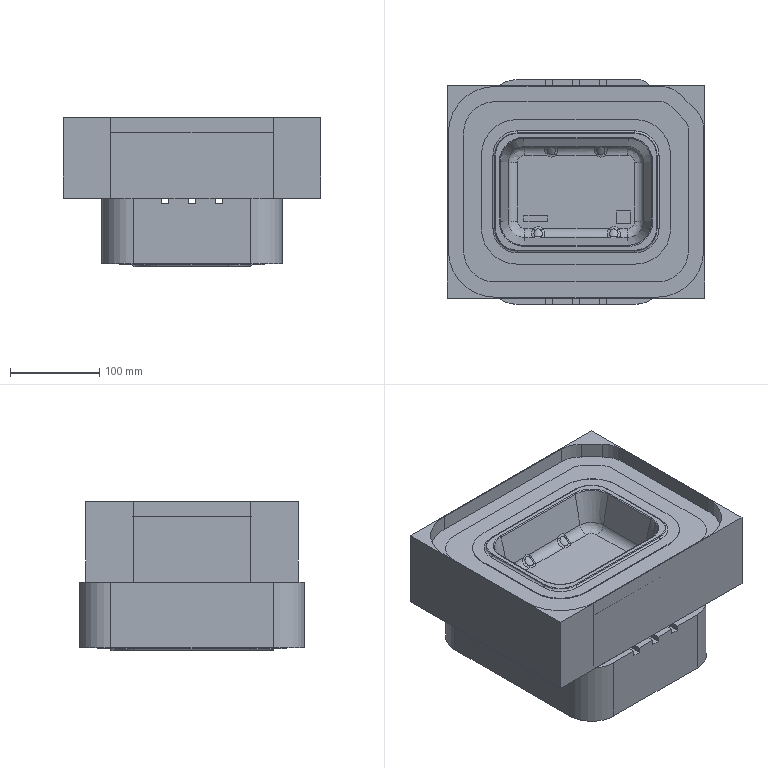NC program | NX | posted with a generic post | part box 287.436 x 251.436 x 167.016 mm
Lines 12631 to 13522 of 118587:
(06 , TOOL : R2)
N25248 M6
N25250 G53
N25252 G17 G0 G90 X-67.849 Y-80.733 S8000 M3 M8
N25254 G43 Z240.5 H0
N25256 Z77.182
N25258 G94 G1 Z74.182 F4500.
N25260 X-69.235 Y-80.679
N25262 X-69.472 Y-80.657
N25264 X-69.58 Y-80.643
N25266 X-70.616 Y-80.526
N25268 X-72.004 Y-80.366
N25270 X-72.391 Y-80.311
N25272 X-74.221 Y-79.965
N25274 X-75.119 Y-79.784
N25276 X-75.413 Y-79.709
N25278 X-75.763 Y-79.619
N25280 X-75.811 Y-79.604
N25282 X-77.051 Y-79.274
N25284 X-77.888 Y-79.04
N25286 X-78.235 Y-78.928
N25288 X-78.245 Y-78.926
N25290 X-80.658 Y-78.075
N25292 X-81.907 Y-77.542
N25294 X-83.423 Y-76.876
N25296 X-83.475 Y-76.849
N25298 X-83.772 Y-76.692
N25300 X-85.849 Y-75.594
N25302 X-86.083 Y-75.464
N25304 X-88.283 Y-74.081
N25306 X-88.617 Y-73.857
N25308 X-88.785 Y-73.734
N25310 X-88.966 Y-73.6
N25312 X-89.258 Y-73.387
N25314 G2 X-96.971 Y-66.118 R37.721
N25316 G1 X-97.247 Y-65.772
N25318 X-97.824 Y-64.992
N25320 X-98.313 Y-64.329
N25322 X-98.78 Y-63.695
N25324 X-99.004 Y-63.36
N25326 X-99.01 Y-63.349
N25328 X-100.389 Y-61.158
N25330 X-100.519 Y-60.924
N25332 X-101.428 Y-59.205
N25334 X-101.799 Y-58.502
N25336 X-102.71 Y-56.425
N25338 X-103. Y-55.733
N25340 X-103.853 Y-53.31
N25342 X-103.965 Y-52.964
N25344 X-104.158 Y-52.277
N25346 X-104.621 Y-50.541
N25348 G2 X-105.291 Y-47.079 R49.648
N25350 G1 X-105.582 Y-44.549
N25352 X-105.601 Y-44.31
N25354 X-105.602 Y-44.28
N25356 X-105.658 Y-42.925
N25358 X-105.706 Y-41.54
N25360 X-105.712 Y-41.194
N25362 X-105.715 Y-40.855
N25364 Y41.187
N25366 X-105.684 Y42.228
N25368 X-105.658 Y42.925
N25370 X-105.602 Y44.28
N25372 X-105.6 Y44.31
N25374 X-105.582 Y44.547
N25376 X-105.568 Y44.656
N25378 X-105.451 Y45.693
N25380 X-105.291 Y47.079
N25382 X-105.236 Y47.466
N25384 X-104.89 Y49.296
N25386 X-104.781 Y49.847
N25388 X-104.709 Y50.194
N25390 X-104.634 Y50.488
N25392 X-104.544 Y50.838
N25394 X-104.343 Y51.579
N25396 X-104.067 Y52.616
N25398 X-103.968 Y52.956
N25400 X-103.853 Y53.31
N25402 X-103.851 Y53.321
N25404 X-103. Y55.733
N25406 X-102.256 Y57.464
N25408 X-101.801 Y58.498
N25410 X-101.774 Y58.55
N25412 X-101.617 Y58.848
N25414 X-100.519 Y60.924
N25416 X-100.389 Y61.158
N25418 X-100.317 Y61.272
N25420 X-100.042 Y61.709
N25422 X-99.448 Y62.656
N25424 X-99.006 Y63.358
N25426 X-98.782 Y63.692
N25428 X-98.659 Y63.86
N25430 X-98.313 Y64.33
N25432 X-98.27 Y64.387
N25434 X-98.077 Y64.649
N25436 X-97.251 Y65.768
N25438 X-96.928 Y66.172
N25440 X-95.186 Y68.195
N25442 X-93.109 Y70.272
N25444 X-91.043 Y72.046
N25446 X-90.664 Y72.349
N25448 X-90.35 Y72.581
N25450 X-88.62 Y73.855
N25452 X-88.284 Y74.079
N25454 X-88.274 Y74.085
N25456 X-87.184 Y74.772
N25458 X-86.635 Y75.118
N25460 X-86.083 Y75.464
N25462 X-85.849 Y75.594
N25464 X-84.13 Y76.503
N25466 X-83.427 Y76.874
N25468 X-81.112 Y77.888
N25470 X-80.658 Y78.075
N25472 X-80.066 Y78.287
N25474 X-78.235 Y78.928
N25476 X-77.888 Y79.04
N25478 X-77.055 Y79.272
N25480 X-75.465 Y79.696
N25482 G2 X-72.004 Y80.366 R49.649
N25484 G1 X-69.473 Y80.657
N25486 X-69.234 Y80.676
N25488 X-67.849 Y80.733
N25490 X-66.465 Y80.781
N25492 X-66.119 Y80.79
N25494 X66.119 Y80.786
N25496 X66.459 Y80.779
N25498 X67.153 Y80.759
N25500 X67.849 Y80.733
N25502 X69.204 Y80.677
N25504 X69.234 Y80.675
N25506 X69.472 Y80.657
N25508 X69.58 Y80.643
N25510 X70.617 Y80.526
N25512 X72.004 Y80.366
N25514 X72.391 Y80.311
N25516 X74.771 Y79.856
N25518 X75.119 Y79.784
N25520 X75.413 Y79.709
N25522 X75.763 Y79.619
N25524 G2 X80.658 Y78.075 R36.873
N25526 G1 X81.112 Y77.888
N25528 X83.475 Y76.849
N25530 X83.773 Y76.692
N25532 X84.787 Y76.156
N25534 X85.849 Y75.594
N25536 X86.082 Y75.465
N25538 X88.283 Y74.081
N25540 X88.617 Y73.857
N25542 X88.785 Y73.734
N25544 X90.675 Y72.34
N25546 X91.096 Y72.003
N25548 X93.109 Y70.272
N25550 X95.186 Y68.195
N25552 X96.971 Y66.118
N25554 X97.051 Y66.018 Z74.18
N25556 X97.246 Y65.773 Z74.182
N25558 X98.313 Y64.329
N25560 X98.78 Y63.695
N25562 X99.004 Y63.36
N25564 X99.01 Y63.349
N25566 X100.389 Y61.158
N25568 X100.518 Y60.926
N25570 X100.882 Y60.234
N25572 X101.066 Y59.887
N25574 X101.799 Y58.502
N25576 X102.256 Y57.464
N25578 X103. Y55.733
N25580 G2 X104.709 Y50.194 R41.459
N25582 G1 X104.78 Y49.848
N25584 X104.917 Y49.156
N25586 X105.242 Y47.425
N25588 X105.291 Y47.079
N25590 X105.582 Y44.549
N25592 X105.601 Y44.31
N25594 X105.658 Y42.925
N25596 X105.684 Y42.232
N25598 X105.715 Y41.194
N25600 X105.712 Y-41.194
N25602 X105.706 Y-41.539
N25604 X105.658 Y-42.925
N25606 X105.602 Y-44.28
N25608 X105.6 Y-44.31
N25610 X105.582 Y-44.547
N25612 X105.568 Y-44.656
N25614 X105.451 Y-45.692
N25616 X105.293 Y-47.065
N25618 X105.242 Y-47.425
N25620 X104.917 Y-49.155
N25622 X104.849 Y-49.502
N25624 X104.709 Y-50.194
N25626 X104.634 Y-50.488
N25628 X104.544 Y-50.838
N25630 X104.529 Y-50.887
N25632 X104.199 Y-52.126
N25634 X103.965 Y-52.964
N25636 X103.853 Y-53.31
N25638 X103.851 Y-53.321
N25640 X103. Y-55.733
N25642 X102.813 Y-56.187
N25644 X101.774 Y-58.55
N25646 X101.617 Y-58.848
N25648 X100.519 Y-60.924
N25650 X100.39 Y-61.157
N25652 X100.317 Y-61.272
N25654 X99.005 Y-63.358
N25656 X98.782 Y-63.692
N25658 X98.659 Y-63.86
N25660 X97.265 Y-65.75
N25662 X97.051 Y-66.018 Z74.18
N25664 X96.971 Y-66.118 Z74.182
N25666 X95.197 Y-68.184
N25668 X93.12 Y-70.261
N25670 X91.097 Y-72.002
N25672 X90.697 Y-72.322
N25674 X89.312 Y-73.344
N25676 X89.307 Y-73.349
N25678 X88.62 Y-73.855
N25680 X88.284 Y-74.08
N25682 X86.083 Y-75.464
N25684 X85.85 Y-75.593
N25686 X85.504 Y-75.777
N25688 X84.13 Y-76.503
N25690 X83.427 Y-76.874
N25692 X82.389 Y-77.331
N25694 X80.658 Y-78.075
N25696 G2 X75.119 Y-79.784 R39.779
N25698 G1 X74.773 Y-79.855
N25700 X74.224 Y-79.964
N25702 X72.393 Y-80.311
N25704 X72.004 Y-80.366
N25706 X69.473 Y-80.657
N25708 X69.234 Y-80.676
N25710 X67.849 Y-80.733
N25712 X67.157 Y-80.759
N25714 X66.465 Y-80.779
N25716 X66.119 Y-80.786
N25718 X-66.112 Y-80.79
N25720 X-66.464 Y-80.781
N25722 X-67.849 Y-80.733
N25724 Y-80.657
N25726 Y-80.447
N25728 X-69.287 Y-80.387
N25730 G2 X-80.658 Y-77.765 R40.675
N25732 X-83.427 Y-76.552 R99.899
N25734 G1 X-85.484 Y-75.465
N25736 X-85.723 Y-75.337
N25738 X-85.85 Y-75.267
N25740 X-85.923 Y-75.227
N25742 G2 X-97.06 Y-65.546 R39.317
N25744 X-101.573 Y-58.302 R39.773
N25746 X-103.766 Y-52.618 R38.865
N25748 G1 X-103.86 Y-52.285
N25750 X-103.943 Y-51.979
N25752 X-104.414 Y-50.194
N25754 X-104.62 Y-49.187
N25756 G2 X-105.372 Y-42.925 R34.123
N25758 G1 X-105.428 Y-41.194
N25760 Y41.194
N25762 X-105.372 Y42.925
N25764 X-105.31 Y44.361
N25766 G2 X-104.954 Y47.425 R61.949
N25768 X-102.597 Y55.948 R40.067
N25770 G1 X-102.094 Y57.118
N25772 X-101.897 Y57.573
N25774 X-101.639 Y58.156
N25776 X-101.531 Y58.4
N25778 X-100.192 Y60.926
N25780 X-100.152 Y60.999
N25782 X-100.043 Y61.172
N25784 G2 X-90.472 Y72.136 R39.166
N25786 X-83.325 Y76.606 R39.555
N25788 X-77.236 Y78.926 R39.766
N25790 X-69.151 Y80.394 R40.837
N25792 G1 X-66.811 Y80.484
N25794 X-66.119 Y80.503
N25796 X66.119
N25798 X67.849 Y80.447
N25800 X69.285 Y80.385
N25802 X69.566 Y80.358
N25804 X70.554 Y80.247
N25806 G2 X76.386 Y79.155 R33.785
N25808 X91.043 Y71.673 R38.456
N25810 G1 X92.915 Y70.062
N25812 G2 X101.944 Y57.464 R38.892
N25814 X104.668 Y48.934 R37.469
N25816 G1 X104.951 Y47.433
N25818 G2 X105.314 Y44.31 R106.611
N25820 G1 X105.404 Y42.054
N25822 X105.429 Y41.041
N25824 X105.428 Y-41.194
N25826 X105.372 Y-42.925
N25828 G2 X103.957 Y-51.925 R36.711
N25830 X101.531 Y-58.4 R36.331
N25832 G1 X100.192 Y-60.926
N25834 X100.152 Y-60.998
N25836 X100.043 Y-61.172
N25838 G2 X94.987 Y-67.99 R42.454
N25840 X83.325 Y-76.606 R39.553
N25842 G1 X82.088 Y-77.15
N25844 G2 X74.112 Y-79.695 R37.012
N25846 X70.7 Y-80.23 R26.407
N25848 G1 X69.58 Y-80.357
N25850 X69.151 Y-80.394
N25852 X66.99 Y-80.478
N25854 X66.276 Y-80.5
N25856 X66.119 Y-80.503
N25858 X-66.119
N25860 X-67.849 Y-80.447
N25862 X-67.839 Y-80.162
N25864 X-69.038 Y-80.115
N25866 X-69.234 Y-80.102
N25868 G2 X-81.796 Y-76.968 R38.488
N25870 X-92.709 Y-69.861 R38.141
N25872 G1 X-94.724 Y-67.849
N25874 G2 X-105.025 Y-44.31 R38.878
N25876 G1 X-105.073 Y-43.271
N25878 X-105.138 Y-41.442
N25880 X-105.145 Y-40.848
N25882 X-105.141 Y41.289
N25884 X-105.087 Y42.925
N25886 G2 X-102.547 Y55.306 R37.867
N25888 X-101.234 Y58.35 R77.91
N25890 X-88.285 Y73.388 R38.937
N25892 X-83.275 Y76.309 R45.716
N25894 G1 X-83.081 Y76.4
N25896 G2 X-67.645 Y80.169 R38.524
N25898 G1 X-66.119 Y80.218
N25900 X66.119
N25902 X67.849 Y80.162
N25904 G2 X76.85 Y78.736 R36.853
N25906 X103.552 Y52.333 R38.75
N25908 G1 X104.12 Y50.194
N25910 G2 X104.734 Y46.923 R63.626
N25912 G1 X105.016 Y44.435
N25914 X105.044 Y43.963
N25916 X105.117 Y42.113
N25918 X105.144 Y41.102
N25920 X105.142 Y-41.288
N25922 X105.081 Y-43.08
N25924 G2 X103.25 Y-53.31 R37.587
N25926 X91.043 Y-71.297 R38.665
N25928 X86.111 Y-74.772 R36.949
N25930 X66.927 Y-80.195 R38.668
N25932 G1 X66.213 Y-80.216
N25934 X66.119 Y-80.218
N25936 X-66.119
N25938 X-67.839 Y-80.162
N25940 X-67.828 Y-79.878
N25942 G2 X-77.591 Y-78.234 R37.518
N25944 X-83.033 Y-76.109 R41.774
N25946 G1 X-83.427 Y-75.907
N25948 X-85.566 Y-74.772
N25950 X-86.543 Y-74.166
N25952 G2 X-92.507 Y-69.659 R36.951
N25954 X-104.805 Y-42.84 R38.466
N25956 G1 X-104.85 Y-41.54
N25958 X-104.859 Y-41.163
N25960 X-104.858 Y41.226
N25962 G2 X-104.725 Y44.474 R55.749
N25964 X-100.832 Y58.502 R38.885
N25966 G1 X-100.043 Y59.994
N25968 X-99.769 Y60.508
N25970 G2 X-85.85 Y74.596 R38.533
N25972 G1 X-85.559 Y74.772
N25974 X-84.692 Y75.239
N25976 G2 X-71.741 Y79.535 R38.091
N25978 X-66.15 Y79.933 R39.099
N25980 G1 X66.088 Y79.934
N25982 X67.765 Y79.88
N25984 G2 X81.004 Y77.001 R37.717
N25986 X96.633 Y65.164 R38.415
N25988 X104.849 Y41.54 R38.518
N25990 G1 X104.859 Y41.163
N25992 X104.858 Y-41.225
N25994 G2 X104.725 Y-44.474 R56.006
N25996 X94.65 Y-67.503 R38.628
N25998 X82.93 Y-76.157 R38.846
N26000 X80.165 Y-77.342 R59.985
N26002 X70.621 Y-79.665 R37.301
N26004 G1 X69.399 Y-79.8
N26006 X68.888 Y-79.834
N26008 X66.864 Y-79.912
N26010 X66.15 Y-79.933
N26012 X-66.088 Y-79.934
N26014 X-67.828 Y-79.878
N26016 X-67.824 Y-79.593
N26018 X-69.153 Y-79.538
N26020 G2 X-78.88 Y-77.495 R37.939
N26022 X-81.617 Y-76.424 R24.696
N26024 G1 X-82.791 Y-75.908
N26026 G2 X-104.432 Y-44.544 R38.287
N26028 G1 X-104.454 Y-44.31
N26030 G2 X-104.573 Y-41.228 R81.56
N26032 G1 X-104.574 Y41.161
N26034 X-104.516 Y42.953
N26036 G2 X-99.466 Y60.464 R38.026
N26038 X-92.428 Y69.337 R39.433
N26040 X-82.518 Y76.028 R38.559
N26042 X-76.972 Y78.112 R37.513
N26044 X-68.888 Y79.549 R38.68
N26046 G1 X-67.877 Y79.591
N26048 X-66.468 Y79.64
N26050 X-66.122 Y79.649
N26052 X66.116
N26054 X67.13 Y79.619
N26056 X67.823 Y79.593
N26058 X69.234 Y79.529
N26060 X70.403 Y79.403
N26062 G2 X80.637 Y76.849 R38.111
N26064 X90.426 Y71.074 R37.642
N26066 X100.82 Y57.895 R38.309
N26068 G1 X101.131 Y57.189
N26070 G2 X103.821 Y48.81 R36.406
N26072 X104.543 Y42.232 R33.916
N26074 G1 X104.573 Y41.227
N26076 X104.574 Y-41.16
N26078 G2 X104.446 Y-44.407 R105.003
N26080 X99.399 Y-60.579 R38.364
N26082 X87.581 Y-73.171 R38.554
N26084 G1 X87.244 Y-73.388
N26086 G2 X81.901 Y-76.299 R36.558
N26088 X70.619 Y-79.378 R37.287
N26090 G1 X69.332 Y-79.521
N26092 X68.888 Y-79.549
N26094 X67.877 Y-79.591
N26096 X67.158 Y-79.618
N26098 X66.122 Y-79.649
N26100 X-66.116
N26102 X-66.462 Y-79.64
N26104 X-67.824 Y-79.593
N26106 X-67.814 Y-79.308
N26108 X-69.21 Y-79.249
N26110 G2 X-80.423 Y-76.626 R39.314
N26112 G1 X-81.366 Y-76.222
N26114 G2 X-90.112 Y-70.964 R36.934
N26116 X-103.801 Y-47.375 R38.037
N26118 X-104.188 Y-43.963 R39.154
N26120 G1 X-104.23 Y-42.962
N26122 X-104.288 Y-41.194
N26124 X-104.287 Y41.194
N26126 X-104.233 Y42.888
N26128 G2 X-101.464 Y55.697 R37.16
N26130 X-93.812 Y67.553 R37.792
N26132 X-91.043 Y70.168 R27.966
N26134 X-77.89 Y77.54 R37.512
N26136 X-74.132 Y78.529 R46.194
N26138 X-66.811 Y79.343 R37.273
N26140 G1 X-66.027 Y79.364
N26142 X66.207 Y79.361
N26144 X67.157 Y79.332
N26146 X67.847 Y79.306
N26148 X69.234 Y79.245
N26150 G2 X97.62 Y62.861 R38.026
N26152 X102.465 Y52.964 R38.023
N26154 X104.172 Y44.284 R40.352
N26156 G1 X104.255 Y42.293
N26158 X104.287 Y41.194
N26160 X104.288 Y-41.194
N26162 X104.233 Y-42.888
N26164 G2 X103.32 Y-49.848 R36.948
N26166 X97.62 Y-62.852 R38.672
N26168 X80.622 Y-76.539 R37.73
N26170 X71.659 Y-78.971 R37.32
N26172 G1 X70.823 Y-79.068
N26174 X69.234 Y-79.244
N26176 X68.897 Y-79.263
N26178 X67.852 Y-79.306
N26180 X67.157 Y-79.333
N26182 X66.027 Y-79.364
N26184 X-66.208 Y-79.361
N26186 X-66.544 Y-79.352
N26188 X-67.814 Y-79.308
N26190 X-67.804 Y-79.023
N26192 X-68.887 Y-78.98
N26194 X-69.232 Y-78.96
N26196 G2 X-82.384 Y-75.465 R37.853
N26198 G1 X-82.624 Y-75.354
N26200 X-83.081 Y-75.123
N26202 G2 X-87.64 Y-72.449 R38.115
N26204 X-103.502 Y-47.425 R37.676
N26206 X-104. Y-41.342 R38.89
N26208 G1 X-104.004 Y-39.183
N26210 X-104.002 Y41.194
N26212 X-103.95 Y42.826
N26214 X-103.906 Y43.909
N26216 G2 X-103.091 Y49.57 R37.858
N26218 X-71.936 Y78.648 R37.729
N26220 X-67.849 Y79.021 R34.091
N26222 G1 X-66.675 Y79.062
N26224 X-65.966 Y79.079
N26226 X66.119 Y79.077
N26228 X67.849 Y79.021
N26230 G2 X72.004 Y78.637 R29.727
N26232 X101.52 Y54.798 R37.727
N26234 X103.903 Y43.963 R38.841
N26236 G1 X103.979 Y42.014
N26238 X104.004 Y41.
N26240 X104.002 Y-41.194
N26242 X103.95 Y-42.826
N26244 G2 X103.562 Y-47.079 R34.249
N26246 X93.812 Y-67.145 R37.913
N26248 X82.394 Y-75.46 R38.484
N26250 X71.936 Y-78.648 R37.859
N26252 X68.889 Y-78.978 R43.378
N26254 G1 X67.032 Y-79.051
N26256 X65.966 Y-79.079
N26258 X-66.119 Y-79.077
N26260 X-67.804 Y-79.023
N26262 X-67.794 Y-78.738
N26264 G2 X-73.734 Y-78.025 R31.327
N26266 G1 X-74.081 Y-77.957
N26268 X-74.773 Y-77.811
N26270 G2 X-82.459 Y-75.118 R38.43
N26272 X-103.713 Y-41.402 R37.457
N26274 G1 X-103.718 Y-41.194
N26276 X-103.719 Y-41.062
N26278 X-103.718 Y41.194
N26280 X-103.667 Y42.763
N26282 G2 X-101.251 Y54.695 R36.677
N26284 X-82.45 Y75.118 R37.518
N26286 X-68.77 Y78.698 R38.049
N26288 G1 X-67.849 Y78.736
N26290 X-66.465 Y78.784
N26292 X-65.905 Y78.794
N26294 X66.119 Y78.793
N26296 X67.849 Y78.736
N26298 G2 X74.426 Y77.888 R32.705
N26300 X100.043 Y57.535 R37.411
N26302 G1 X100.53 Y56.425
N26304 G2 X103.687 Y42.232 R36.678
N26306 G1 X103.719 Y41.062
N26308 X103.715 Y-41.33
N26310 G2 X103.567 Y-44.593 R79.654
N26312 X82.334 Y-75.173 R37.389
N26314 G1 X81.35 Y-75.605
N26316 G2 X67.157 Y-78.762 R37.124
N26318 G1 X66.255 Y-78.79
N26320 X66.119 Y-78.793
N26322 X-66.119
N26324 X-67.794 Y-78.738
N26326 X-67.783 Y-78.453
N26328 G2 X-77.729 Y-76.69 R35.996
N26330 G1 X-79.619 Y-76.023
N26332 X-80.022 Y-75.867
N26334 X-81.233 Y-75.347
N26336 G2 X-89.658 Y-70.23 R36.563
N26338 G1 X-91.498 Y-68.65
N26340 G2 X-103.412 Y-41.886 R37.175
N26342 G1 X-103.434 Y-41.123
N26344 X-103.431 Y41.268
N26346 X-103.384 Y42.699
N26348 G2 X-100.353 Y56.116 R36.296
N26350 X-91.389 Y68.736 R36.847
N26352 X-69.071 Y78.397 R37.292
N26354 G1 X-67.625 Y78.459
N26356 X-66.119 Y78.508
N26358 X66.119
N26360 X67.849 Y78.45
N26362 G2 X82.888 Y74.58 R36.659
N26364 X102.377 Y50.104 R36.976
N26366 G1 X102.442 Y49.848
N26368 X102.467 Y49.75
N26370 G2 X103.402 Y42.232 R36.493
N26372 G1 X103.434 Y41.122
N26374 X103.432 Y-41.267
N26376 X103.375 Y-42.925
N26378 G2 X102.436 Y-49.879 R36.895
N26380 X82.276 Y-74.885 R37.19
N26382 G1 X81.35 Y-75.294
N26384 G2 X67.264 Y-78.473 R36.499
N26386 G1 X66.119 Y-78.508
N26388 X-66.119
N26390 X-67.783 Y-78.453
N26392 Y-78.168
N26394 G2 X-73.942 Y-77.403 R31.517
N26396 X-81.003 Y-75.136 R35.593
N26398 X-94.812 Y-64.694 R36.447
N26400 G1 X-94.963 Y-64.516
N26402 G2 X-103.09 Y-42.925 R36.737
N26404 G1 X-103.139 Y-41.54
N26406 X-103.149 Y-41.194
N26408 X-103.148 Y41.205
N26410 G2 X-103.008 Y44.46 R86.936
N26412 X-102.229 Y49.502 R38.617
N26414 X-99.602 Y57.118 R37.192
N26416 X-87.157 Y71.735 R36.838
N26418 X-77.618 Y76.427 R36.436
N26420 X-75.204 Y77.111 R26.715
N26422 G1 X-74.734 Y77.234
N26424 G2 X-68.643 Y78.133 R36.077
N26426 G1 X-67.849 Y78.165
N26428 X-66.485 Y78.214
N26430 X-66.119 Y78.224
N26432 X66.108
N26434 X67.116 Y78.193
N26436 X67.783 Y78.168
N26438 G2 X82.418 Y74.504 R36.718
N26440 X103.117 Y42.232 R36.785
N26442 G1 X103.148 Y41.194
N26444 X103.149 Y-41.194
N26446 X103.139 Y-41.54
N26448 X103.101 Y-42.637
N26450 G2 X102.159 Y-49.809 R36.984
N26452 X67.201 Y-78.19 R36.824
N26454 G1 X66.129 Y-78.223
N26456 X-66.108 Y-78.224
N26458 X-66.446 Y-78.215
N26460 X-67.783 Y-78.168
N26462 X-67.773 Y-77.883
N26464 G2 X-79.273 Y-75.543 R35.553
N26466 G1 X-79.487 Y-75.465
N26468 X-79.619 Y-75.413
N26470 X-80.658 Y-74.975
N26472 G2 X-101.854 Y-49.848 R36.401
N26474 X-102.805 Y-42.925 R34.76
N26476 G1 X-102.863 Y-41.194
N26478 Y41.194
N26480 X-102.819 Y42.572
N26482 G2 X-93.466 Y65.823 R36.441
N26484 X-67.857 Y77.88 R36.454
N26486 G1 X-66.467 Y77.929
N26488 X-66.12 Y77.939
N26490 X66.117 Y77.938
N26492 G2 X69.234 Y77.812 R50.755
N26494 X101.326 Y51.823 R36.562
N26496 X102.831 Y42.254 R35.758
N26498 G1 X102.862 Y41.246
N26500 X102.863 Y41.194
N26502 Y-41.194
N26504 G2 X102.729 Y-44.394 R97.577
N26506 X101.937 Y-49.502 R36.746
N26508 X96.255 Y-62.31 R36.8
N26510 X93.466 Y-65.823 R34.695
N26512 X79.152 Y-75.586 R36.834
N26514 X67.16 Y-77.906 R36.508
N26516 G1 X66.12 Y-77.938
N26518 X-66.117
N26520 X-66.462 Y-77.929
N26522 X-67.773 Y-77.883
N26524 X-67.764 Y-77.598
N26526 G2 X-71.98 Y-77.195 R28.768
N26528 X-88.665 Y-69.926 R36.463
N26530 X-102.52 Y-42.925 R36.147
N26532 G1 X-102.577 Y-41.194
N26534 Y41.194
N26536 X-102.536 Y42.509
N26538 G2 X-92.815 Y66.118 R36.199
N26540 X-68.89 Y77.551 R36.399
N26542 G1 X-67.851 Y77.595
N26544 X-66.718 Y77.635
N26546 X-66.007 Y77.653
N26548 X66.119 Y77.652
N26550 X67.848 Y77.595
N26552 G2 X79.335 Y75.217 R35.426
N26554 X99.005 Y57.059 R36.173
N26556 X100.166 Y54.348 R53.776
N26558 X102.546 Y42.232 R35.771
N26560 G1 X102.575 Y41.302
N26562 X102.577 Y41.194
N26564 Y-41.194
N26566 G2 X102.449 Y-44.327 R66.803
N26568 X101.644 Y-49.502 R36.419
N26570 X68.89 Y-77.551 R36.281
N26572 G1 X67.851 Y-77.595
N26574 X67.157 Y-77.621
N26576 X66.007 Y-77.653
N26578 X-66.227 Y-77.65
N26580 X-66.465 Y-77.643
N26582 X-67.764 Y-77.598
N26584 X-67.753 Y-77.313
N26586 G2 X-77.087 Y-75.701 R35.081
N26588 X-102.189 Y-43.963 R35.976
N26590 G1 X-102.243 Y-42.701
N26592 X-102.292 Y-41.194
N26594 X-102.291 Y41.194
N26596 X-102.253 Y42.446
N26598 G2 X-93.055 Y65.426 R35.878
N26600 X-68.814 Y77.269 R36.069
N26602 G1 X-67.849 Y77.31
N26604 X-67.372 Y77.327
N26606 X-66.119 Y77.367
N26608 X66.119 Y77.366
N26610 X67.849 Y77.309
N26612 G2 X84.12 Y72.637 R35.716
N26614 X102.267 Y42.033 R35.938
N26616 G1 X102.293 Y41.02
N26618 X102.292 Y-41.194
N26620 X102.252 Y-42.447
N26622 G2 X100.825 Y-51.49 R34.902
N26624 X67.012 Y-77.341 R35.963
N26626 G1 X65.946 Y-77.368
N26628 X-66.119 Y-77.367
N26630 X-67.753 Y-77.313
N26632 X-67.743 Y-77.028
N26634 G2 X-80.658 Y-74.042 R34.988
N26636 X-101.275 Y-48.464 R35.613
N26638 X-101.955 Y-42.76 R31.107
N26640 G1 X-102.007 Y-41.194
N26642 X-102.004 Y41.31
N26644 G2 X-101.876 Y44.31 R90.531
N26646 X-66.591 Y77.069 R35.708
N26648 G1 X-65.885 Y77.083
N26650 X66.119 Y77.081
N26652 X67.849 Y77.024
N26654 G2 X79.775 Y74.426 R35.182
N26656 X99.774 Y53.748 R35.534
N26658 X101.98 Y42.092 R35.907
N26660 G1 X102.008 Y41.081
N26662 X102.005 Y-41.309
N26664 G2 X98.335 Y-57.117 R35.854
N26666 X66.949 Y-77.057 R35.686
N26668 G1 X66.235 Y-77.079
N26670 X66.119 Y-77.081
N26672 X-66.119 Y-77.082
N26674 X-67.743 Y-77.028
N26676 X-67.733 Y-76.743
N26678 G2 X-81.847 Y-73.192 R35.173
N26680 X-92.428 Y-65.283 R35.493
N26682 X-95.712 Y-61.094 R36.01
N26684 X-101.664 Y-42.925 R35.248
N26686 G1 X-101.723 Y-41.143
N26688 X-101.721 Y41.247
N26690 X-101.701 Y41.886
N26692 G2 X-68.687 Y76.704 R35.413
N26694 G1 X-67.849 Y76.739
N26696 X-66.119 Y76.798
N26698 X66.119 Y76.797
N26700 G2 X71.311 Y76.427 R37.706
N26702 X101.701 Y41.886 R35.366
N26704 G1 X101.722 Y41.194
N26706 X101.723 Y41.143
N26708 X101.722 Y-41.247
N26710 G2 X100.777 Y-49.461 R37.559
N26712 X67.157 Y-76.766 R35.415
N26714 G1 X66.172 Y-76.796
N26716 X66.119 Y-76.797
N26718 X-66.119
N26720 X-66.465 Y-76.788
N26722 X-67.733 Y-76.743
N26724 X-67.723 Y-76.459
N26726 G2 X-71.6 Y-76.1 R33.297
N26728 X-93.707 Y-63.349 R35.3
N26730 X-101.428 Y-41.54 R35.324
N26732 G1 X-101.438 Y-41.194
N26734 Y41.183
N26736 X-101.416 Y41.886
N26738 G2 X-67.849 Y76.454 R35.102
N26740 G1 X-66.467 Y76.503
N26742 X-66.12 Y76.513
N26744 X66.117
N26746 X67.135 Y76.481
N26748 G2 X100.975 Y46.971 R35.07
N26750 X101.405 Y42.232 R35.119
N26752 G1 X101.437 Y41.205
N26754 X101.438 Y-41.182
N26756 X101.364 Y-43.271
N26758 G2 X93.466 Y-63.631 R34.957
N26760 X67.181 Y-76.48 R35.069
N26762 G1 X66.12 Y-76.513
N26764 X-66.117
N26766 X-66.463 Y-76.503
N26768 X-67.723 Y-76.459
N26770 X-67.713 Y-76.174
N26772 G2 X-71.607 Y-75.811 R34.352
N26774 G1 X-71.946 Y-75.753
N26776 G2 X-88.204 Y-68.471 R34.839
N26778 X-101.093 Y-42.939 R34.849
N26780 G1 X-101.152 Y-41.194
N26782 Y41.194
N26784 X-101.133 Y41.835
N26786 G2 X-67.852 Y76.169 R34.817
N26788 G1 X-66.048 Y76.228
N26790 X66.178 Y76.225
N26792 G2 X69.234 Y76.092 R73.05
N26794 X100.677 Y47.02 R34.826
N26796 X101.119 Y42.269 R31.472
N26798 G1 X101.15 Y41.263
N26800 X101.152 Y41.194
N26802 Y-41.194
N26804 X101.082 Y-43.191
N26806 G2 X67.16 Y-76.195 R34.815
N26808 G1 X66.048 Y-76.228
N26810 X-66.187 Y-76.226
N26812 X-66.465 Y-76.218
N26814 X-67.713 Y-76.174
N26816 X-67.703 Y-75.889
N26818 G2 X-81.004 Y-72.645 R34.341
N26820 X-100.808 Y-42.925 R34.515
N26822 G1 X-100.866 Y-41.194
N26824 Y41.194
N26826 X-100.838 Y42.131
N26828 G2 X-76.555 Y74.375 R34.557
N26830 G1 X-76.383 Y74.426
N26832 G2 X-67.849 Y75.883 R33.405
N26834 G1 X-66.119 Y75.941
N26836 X66.119
N26838 G2 X71.311 Y75.564 R38.518
N26840 X89.858 Y66.664 R34.588
N26842 X100.831 Y42.328 R34.546
N26844 G1 X100.866 Y41.194
N26846 Y-41.194
N26848 G2 X100.731 Y-44.31 R47.789
N26850 X67.157 Y-75.91 R34.551
N26852 G1 X65.987 Y-75.942
N26854 X-66.119 Y-75.941
N26856 X-67.703 Y-75.889
N26858 X-67.693 Y-75.604
N26860 G2 X-71.311 Y-75.276 R26.887
N26862 X-94.605 Y-60.699 R34.259
N26864 X-100.523 Y-42.925 R34.135
N26866 G1 X-100.582 Y-41.194
N26868 X-100.581 Y41.194
N26870 X-100.555 Y42.067
N26872 G2 X-67.849 Y75.598 R34.251
N26874 G1 X-66.119 Y75.657
N26876 X66.119 Y75.656
N26878 X67.644 Y75.606
N26880 G2 X83.268 Y71.151 R34.058
N26882 X94.851 Y60.325 R34.161
N26884 X100.549 Y42.232 R34.095
N26886 G1 X100.582 Y41.041
N26888 Y-41.194
N26890 X100.522 Y-42.925
N26892 G2 X90.004 Y-66.114 R34.197
N26894 X68.796 Y-75.556 R34.44
N26896 G1 X67.157 Y-75.625
N26898 X66.277 Y-75.652
N26900 X66.119 Y-75.656
N26902 X-66.119 Y-75.657
N26904 X-67.693 Y-75.604
N26906 X-67.683 Y-75.319
N26908 G2 X-98.863 Y-51.091 R33.93
N26910 X-100.243 Y-42.778 R33.243
N26912 G1 X-100.297 Y-41.102
N26914 X-100.294 Y41.29
N26916 G2 X-99.893 Y46.537 R38.775
N26918 X-66.571 Y75.359 R34.021
N26920 G1 X-66.214 Y75.37
N26922 X-66.119 Y75.371
N26924 X66.119
N26926 X67.703 Y75.318
N26928 G2 X100.268 Y42.111 R33.935
N26930 G1 X100.297 Y41.102
N26932 X100.295 Y-41.289
N26934 G2 X87.504 Y-67.927 R34.028
N26936 X68.008 Y-75.306 R34.016
N26938 G1 X66.119 Y-75.371
N26940 X-66.119
N26942 X-67.683 Y-75.319
N26944 X-67.673 Y-75.034
N26946 G2 X-99.952 Y-42.925 R33.63
N26948 G1 X-99.992 Y-41.834
N26950 X-100.012 Y-41.194
N26952 Y-41.163
N26954 X-100.011 Y41.227
N26956 G2 X-97.62 Y53.795 R33.776
N26958 X-66.507 Y75.076 R33.718
N26960 G1 X-66.151 Y75.087
N26962 X-66.119
N26964 X66.119 Y75.086
N26966 X67.095 Y75.056
N26968 G2 X99.979 Y42.232 R33.642
N26970 G1 X100.012 Y41.194
N26972 Y41.163
N26974 Y-41.194
N26976 G2 X99.118 Y-49.043 R35.121
N26978 X67.157 Y-75.054 R33.703
N26980 G1 X66.151 Y-75.086
N26982 X66.119 Y-75.087
N26984 X-66.119
N26986 X-66.425 Y-75.078
N26988 X-67.673 Y-75.034
N26990 X-67.663 Y-74.749
N26992 G2 X-81.02 Y-71.373 R33.227
N26994 X-99.015 Y-48.133 R33.351
N26996 X-99.727 Y-41.194 R34.656
N26998 G1 X-99.726 Y41.194
N27000 G2 X-98.842 Y48.973 R34.151
N27002 X-66.468 Y74.792 R33.461
N27004 G1 X-66.122 Y74.802
N27006 X66.116
N27008 X67.154 Y74.769
N27010 G2 X99.582 Y44.31 R33.389
N27012 G1 X99.621 Y43.888
N27014 X99.694 Y42.232
N27016 X99.726 Y41.227
N27018 Y41.194
N27020 X99.727 Y-41.194
N27022 G2 X98.841 Y-48.973 R34.87
N27024 X67.16 Y-74.769 R33.433